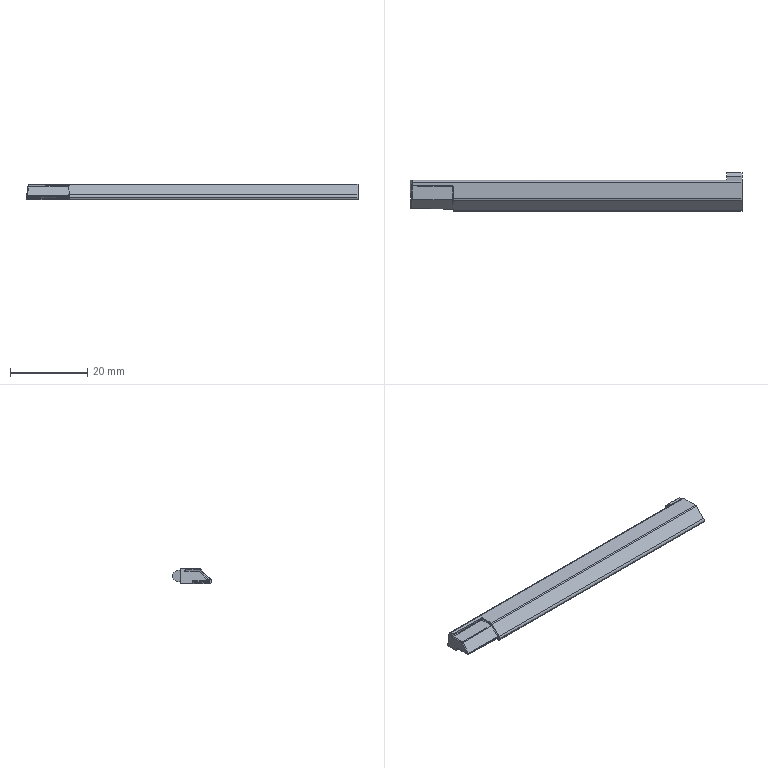Part | Creo | 1 solid | 52 faces | box 85.89 x 10 x 4 mm | volume 2284 mm3 | cylinder 22 | plane 19 | spline 6 | sphere 5 | commonest cylinder face diameters 0.402 x17 1 x4 2 x1